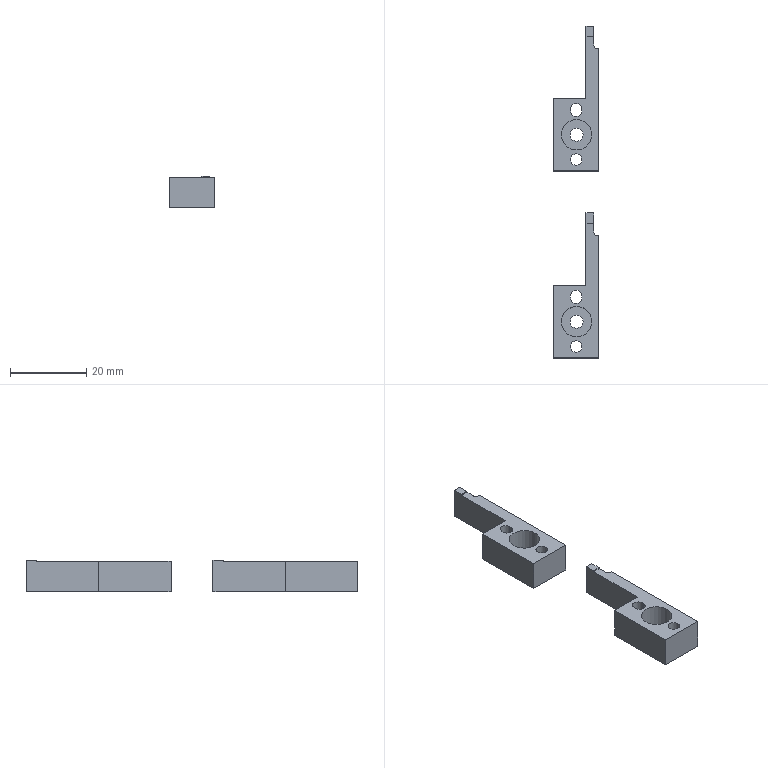CAM job | NX | 3-axis milling, drilling | part box 11.9 x 87 x 8.25 mm | stock box 16.9 x 91 x 12 mm
Tools:
number,name,description,diameter,corner_radius,flute_length,length,flutes
18,D2,平底铣刀-粗,2.0,0.0,50.0,75.0,2
4,D4,平底铣刀-粗,4.0,0.0,25.0,75.0,2
9,D10,平底铣刀-粗,10.0,0.0,35.0,75.0,2
19,D2-J,平底铣刀-精,2.0,0.0,50.0,75.0,2
11,D4-J,平底铣刀-精,4.0,0.0,50.0,75.0,2
7,D6-J,平底铣刀-精,6.0,0.0,25.0,75.0,2
10,D10-J,平底铣刀-精,10.0,0.0,35.0,75.0,2
2,D6倒角刀,倒角刀,6.0,0.0,3.0,25.0,2
13,ZT3.4,钻头,3.4,0.0,35.0,50.0,2
17,ZT2.9,Drilling Tool,2.9,0.0,35.0,50.0,2
Operations:
program,operation,operation_type,tool,method,geometry_group,spindle_rpm,surface_speed,feed_per_tooth,feed_cut,feed_plunge,cut_length_mm,path_length_mm,cut_time_min,machine_time_min
A,顶面,FaceMilling,D10-J,侧刃精光-切深K-步距G,W-A,8000.0,251.327,0.0625,1000.0,100.0,315.95,351.95,0.3159,0.3195
A,型腔铣开粗-中_COPY,CavityMilling,D10,分层开粗-切深K-步距G,W-A,8000.0,251.32,0.25,4000.0,100.0,11097.43,11481.98,2.774,2.831
A,打点-深0.8,Operation,D6倒角刀,NONE,W-A,8000.0,150.796,0.0312,500.0,90.0,10.8,214.538,0.0216,0.042
A,通孔-精孔3.0预钻,Operation,ZT2.9,NONE,W-A,3200.0,29.154,0.0312,200.0,90.0,51.349,257.007,0.2567,0.2773
A,沉头孔-钻孔0段,Operation,ZT3.4,NONE,W-A,2800.0,29.908,0.0357,200.0,90.0,24.043,138.596,0.1202,0.1317
A,底壁粗_1,VolumeBased25DMillingOperation,D10,METHOD,W-A,6000.0,113.0,0.2083,3500.0,100.0,283.176,410.779,0.0809,0.0937
A,通腰槽粗_1,VolumeBased25DMillingOperation,D2,METHOD,W-A,6000.0,37.699,0.05,600.0,100.0,707.48,851.975,1.179,1.194
A,铣孔开粗D2_1,CylinderMilling,D2,NONE,W-A,8000.0,50.266,0.0312,500.0,100.0,257.758,403.758,0.5155,0.5301
A,铣孔开粗D4_1,CylinderMilling,D4,NONE,W-A,8000.0,100.531,0.075,1200.0,100.0,553.293,694.293,0.4611,0.4752
A,外形侧面,ZLevelMilling,D2-J,METHOD,W-A,9000.0,56.549,0.0833,1500.0,80.0,2312.762,2565.407,1.543,1.568
A,仅选体,SurfaceContour,D6倒角刀,METHOD,W-A,8000.0,150.796,0.1875,3000.0,100.0,270.748,605.372,0.0902,0.1237
A,钻倒角_1,Operation,D6倒角刀,METHOD,W-A,8000.0,150.796,0.0312,500.0,0.0,9.6,111.792,0.0192,0.0294
A,铣倒角_1,PlanarMilling,D6倒角刀,NONE,W-A,8000.0,150.796,0.0312,500.0,100.0,67.936,191.596,0.1359,0.1482
A,腰槽精_1,VolumeBased25DMillingOperation,D2-J,METHOD,W-A,6000.0,113.0,0.0167,200.0,100.0,119.69,471.077,0.5985,0.6336
A,铣孔精光D4_1,CylinderMilling,D4-J,精光步距切深关,W-A,8000.0,100.531,0.0312,500.0,100.0,73.089,214.089,0.1462,0.1603
A,底精_1,VolumeBased25DMillingOperation,D6-J,METHOD,W-A,6000.0,113.0,0.2083,1200.0,100.0,290.232,417.732,0.2419,0.2546
A,底侧精_3,VolumeBased25DMillingOperation,D6-J,METHOD,W-A,6000.0,113.0,0.2083,1200.0,100.0,29.003,162.384,0.0242,0.0375
A,外形半精_2,VolumeBased25DMillingOperation,D6-J,METHOD,W-A,8000.0,251.327,0.0625,1000.0,100.0,242.823,406.54,0.2428,0.2592